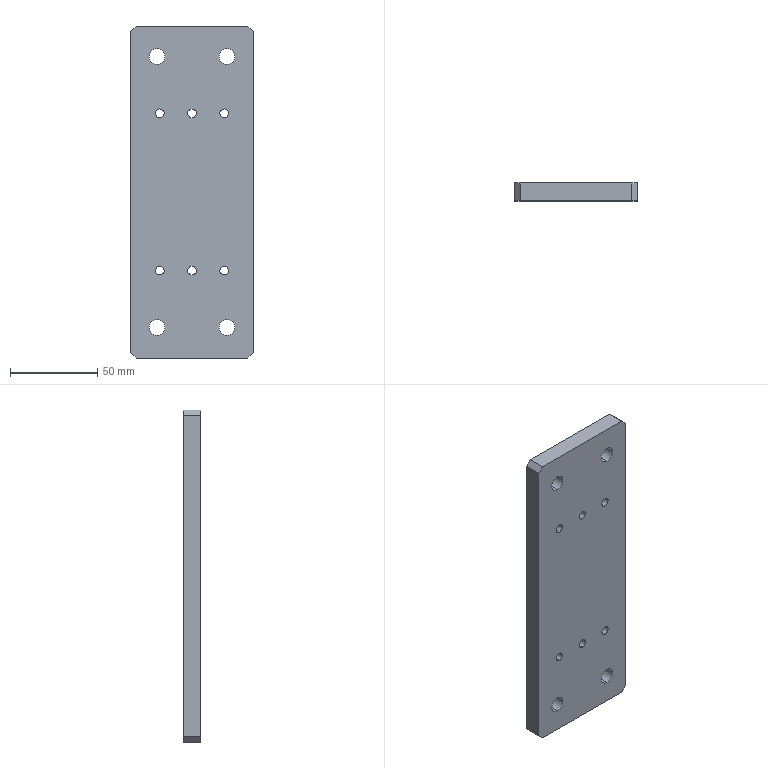Part | SolidWorks | features HoleWzd 2, Chamfer 1, Extrusion 1 | 1 solid | 30 faces | box 70 x 10 x 190 mm | volume 129097 mm3 | cylinder 20 | plane 10 | commonest cylinder face diameters 5 x12 9 x8
STEP:
#1=CARTESIAN_POINT('',(-20.,0.,-82.));
#2=VERTEX_POINT('',#1);
#3=CARTESIAN_POINT('',(-20.,0.,-73.));
#4=VERTEX_POINT('',#3);
#5=CARTESIAN_POINT('',(-20.,0.,-77.5));
#6=DIRECTION('',(0.,1.,0.));
#7=DIRECTION('',(0.,0.,1.));
#8=AXIS2_PLACEMENT_3D('',#5,#6,#7);
#9=CIRCLE('',#8,4.5);
#10=EDGE_CURVE('',#2,#4,#9,.T.);
#11=ORIENTED_EDGE('',*,*,#10,.F.);
#12=CARTESIAN_POINT('',(-20.,10.,-82.));
#13=VERTEX_POINT('',#12);
#14=CARTESIAN_POINT('',(-20.,10.,-82.));
#15=DIRECTION('',(0.,1.,0.));
#16=VECTOR('',#15,1000.);
#17=LINE('',#14,#16);
#18=EDGE_CURVE('',#2,#13,#17,.T.);
#19=ORIENTED_EDGE('',*,*,#18,.T.);
#20=CARTESIAN_POINT('',(-20.,10.,-73.));
#21=VERTEX_POINT('',#20);
#22=CARTESIAN_POINT('',(-20.,10.,-77.5));
#23=DIRECTION('',(0.,1.,0.));
#24=DIRECTION('',(0.,0.,1.));
#25=AXIS2_PLACEMENT_3D('',#22,#23,#24);
#26=CIRCLE('',#25,4.5);
#27=EDGE_CURVE('',#13,#21,#26,.T.);
#28=ORIENTED_EDGE('',*,*,#27,.T.);
#29=CARTESIAN_POINT('',(-20.,10.,-73.));
#30=DIRECTION('',(0.,1.,0.));
#31=VECTOR('',#30,1000.);
#32=LINE('',#29,#31);
#33=EDGE_CURVE('',#4,#21,#32,.T.);
#34=ORIENTED_EDGE('',*,*,#33,.F.);
#35=EDGE_LOOP('',(#11,#19,#28,#34));
#36=FACE_OUTER_BOUND('',#35,.T.);
#37=CARTESIAN_POINT('',(-20.,10.,-77.5));
#38=DIRECTION('',(0.,1.,0.));
#39=DIRECTION('',(0.,0.,1.));
#40=AXIS2_PLACEMENT_3D('',#37,#38,#39);
#41=CYLINDRICAL_SURFACE('',#40,4.5);
#42=ADVANCED_FACE('',(#36),#41,.F.);
#43=CARTESIAN_POINT('',(20.,0.,-82.));
#44=VERTEX_POINT('',#43);
#45=CARTESIAN_POINT('',(20.,0.,-73.));
#46=VERTEX_POINT('',#45);
#47=CARTESIAN_POINT('',(20.,0.,-77.5));
#48=DIRECTION('',(0.,1.,0.));
#49=DIRECTION('',(0.,0.,1.));
#50=AXIS2_PLACEMENT_3D('',#47,#48,#49);
#51=CIRCLE('',#50,4.5);
#52=EDGE_CURVE('',#44,#46,#51,.T.);
#53=ORIENTED_EDGE('',*,*,#52,.F.);
#54=CARTESIAN_POINT('',(20.,10.,-82.));
#55=VERTEX_POINT('',#54);
#56=CARTESIAN_POINT('',(20.,10.,-82.));
#57=DIRECTION('',(0.,1.,0.));
#58=VECTOR('',#57,1000.);
#59=LINE('',#56,#58);
#60=EDGE_CURVE('',#44,#55,#59,.T.);
#61=ORIENTED_EDGE('',*,*,#60,.T.);
#62=CARTESIAN_POINT('',(20.,10.,-73.));
#63=VERTEX_POINT('',#62);
#64=CARTESIAN_POINT('',(20.,10.,-77.5));
#65=DIRECTION('',(0.,1.,0.));
#66=DIRECTION('',(0.,0.,1.));
#67=AXIS2_PLACEMENT_3D('',#64,#65,#66);
#68=CIRCLE('',#67,4.5);
#69=EDGE_CURVE('',#55,#63,#68,.T.);
#70=ORIENTED_EDGE('',*,*,#69,.T.);
#71=CARTESIAN_POINT('',(20.,10.,-73.));
#72=DIRECTION('',(0.,1.,0.));
#73=VECTOR('',#72,1000.);
#74=LINE('',#71,#73);
#75=EDGE_CURVE('',#46,#63,#74,.T.);
#76=ORIENTED_EDGE('',*,*,#75,.F.);
#77=EDGE_LOOP('',(#53,#61,#70,#76));
#78=FACE_OUTER_BOUND('',#77,.T.);
#79=CARTESIAN_POINT('',(20.,10.,-77.5));
#80=DIRECTION('',(0.,1.,0.));
#81=DIRECTION('',(0.,0.,1.));
#82=AXIS2_PLACEMENT_3D('',#79,#80,#81);
#83=CYLINDRICAL_SURFACE('',#82,4.5);
#84=ADVANCED_FACE('',(#78),#83,.F.);
#85=CARTESIAN_POINT('',(20.,0.,73.));
#86=VERTEX_POINT('',#85);
#87=CARTESIAN_POINT('',(20.,0.,82.));
#88=VERTEX_POINT('',#87);
#89=CARTESIAN_POINT('',(20.,0.,77.5));
#90=DIRECTION('',(0.,1.,0.));
#91=DIRECTION('',(0.,0.,1.));
#92=AXIS2_PLACEMENT_3D('',#89,#90,#91);
#93=CIRCLE('',#92,4.5);
#94=EDGE_CURVE('',#86,#88,#93,.T.);
#95=ORIENTED_EDGE('',*,*,#94,.F.);
#96=CARTESIAN_POINT('',(20.,10.,73.));
#97=VERTEX_POINT('',#96);
#98=CARTESIAN_POINT('',(20.,10.,73.));
#99=DIRECTION('',(0.,1.,0.));
#100=VECTOR('',#99,1000.);
#101=LINE('',#98,#100);
#102=EDGE_CURVE('',#86,#97,#101,.T.);
#103=ORIENTED_EDGE('',*,*,#102,.T.);
#104=CARTESIAN_POINT('',(20.,10.,82.));
#105=VERTEX_POINT('',#104);
#106=CARTESIAN_POINT('',(20.,10.,77.5));
#107=DIRECTION('',(0.,1.,0.));
#108=DIRECTION('',(0.,0.,1.));
#109=AXIS2_PLACEMENT_3D('',#106,#107,#108);
#110=CIRCLE('',#109,4.5);
#111=EDGE_CURVE('',#97,#105,#110,.T.);
#112=ORIENTED_EDGE('',*,*,#111,.T.);
#113=CARTESIAN_POINT('',(20.,10.,82.));
#114=DIRECTION('',(0.,1.,0.));
#115=VECTOR('',#114,1000.);
#116=LINE('',#113,#115);
#117=EDGE_CURVE('',#88,#105,#116,.T.);
#118=ORIENTED_EDGE('',*,*,#117,.F.);
#119=EDGE_LOOP('',(#95,#103,#112,#118));
#120=FACE_OUTER_BOUND('',#119,.T.);
#121=CARTESIAN_POINT('',(20.,10.,77.5));
#122=DIRECTION('',(0.,1.,0.));
#123=DIRECTION('',(0.,0.,1.));
#124=AXIS2_PLACEMENT_3D('',#121,#122,#123);
#125=CYLINDRICAL_SURFACE('',#124,4.5);
#126=ADVANCED_FACE('',(#120),#125,.F.);
#127=CARTESIAN_POINT('',(-20.,0.,73.));
#128=VERTEX_POINT('',#127);
#129=CARTESIAN_POINT('',(-20.,0.,82.));
#130=VERTEX_POINT('',#129);
#131=CARTESIAN_POINT('',(-20.,0.,77.5));
#132=DIRECTION('',(0.,1.,0.));
#133=DIRECTION('',(0.,0.,1.));
#134=AXIS2_PLACEMENT_3D('',#131,#132,#133);
#135=CIRCLE('',#134,4.5);
#136=EDGE_CURVE('',#128,#130,#135,.T.);
#137=ORIENTED_EDGE('',*,*,#136,.F.);
#138=CARTESIAN_POINT('',(-20.,10.,73.));
#139=VERTEX_POINT('',#138);
#140=CARTESIAN_POINT('',(-20.,10.,73.));
#141=DIRECTION('',(0.,1.,0.));
#142=VECTOR('',#141,1000.);
#143=LINE('',#140,#142);
#144=EDGE_CURVE('',#128,#139,#143,.T.);
#145=ORIENTED_EDGE('',*,*,#144,.T.);
#146=CARTESIAN_POINT('',(-20.,10.,82.));
#147=VERTEX_POINT('',#146);
#148=CARTESIAN_POINT('',(-20.,10.,77.5));
#149=DIRECTION('',(0.,1.,0.));
#150=DIRECTION('',(0.,0.,1.));
#151=AXIS2_PLACEMENT_3D('',#148,#149,#150);
#152=CIRCLE('',#151,4.5);
#153=EDGE_CURVE('',#139,#147,#152,.T.);
#154=ORIENTED_EDGE('',*,*,#153,.T.);
#155=CARTESIAN_POINT('',(-20.,10.,82.));
#156=DIRECTION('',(0.,1.,0.));
#157=VECTOR('',#156,1000.);
#158=LINE('',#155,#157);
#159=EDGE_CURVE('',#130,#147,#158,.T.);
#160=ORIENTED_EDGE('',*,*,#159,.F.);
#161=EDGE_LOOP('',(#137,#145,#154,#160));
#162=FACE_OUTER_BOUND('',#161,.T.);
#163=CARTESIAN_POINT('',(-20.,10.,77.5));
#164=DIRECTION('',(0.,1.,0.));
#165=DIRECTION('',(0.,0.,1.));
#166=AXIS2_PLACEMENT_3D('',#163,#164,#165);
#167=CYLINDRICAL_SURFACE('',#166,4.5);
#168=ADVANCED_FACE('',(#162),#167,.F.);
#169=CARTESIAN_POINT('',(18.5,0.,-47.5));
#170=VERTEX_POINT('',#169);
#171=CARTESIAN_POINT('',(18.5,0.,-42.5));
#172=VERTEX_POINT('',#171);
#173=CARTESIAN_POINT('',(18.5,0.,-45.));
#174=DIRECTION('',(0.,1.,0.));
#175=DIRECTION('',(0.,0.,1.));
#176=AXIS2_PLACEMENT_3D('',#173,#174,#175);
#177=CIRCLE('',#176,2.5);
#178=EDGE_CURVE('',#170,#172,#177,.T.);
#179=ORIENTED_EDGE('',*,*,#178,.F.);
#180=CARTESIAN_POINT('',(18.5,10.,-47.5));
#181=VERTEX_POINT('',#180);
#182=CARTESIAN_POINT('',(18.5,10.,-47.5));
#183=DIRECTION('',(0.,1.,0.));
#184=VECTOR('',#183,1000.);
#185=LINE('',#182,#184);
#186=EDGE_CURVE('',#170,#181,#185,.T.);
#187=ORIENTED_EDGE('',*,*,#186,.T.);
#188=CARTESIAN_POINT('',(18.5,10.,-42.5));
#189=VERTEX_POINT('',#188);
#190=CARTESIAN_POINT('',(18.5,10.,-45.));
#191=DIRECTION('',(0.,1.,0.));
#192=DIRECTION('',(0.,0.,1.));
#193=AXIS2_PLACEMENT_3D('',#190,#191,#192);
#194=CIRCLE('',#193,2.5);
#195=EDGE_CURVE('',#181,#189,#194,.T.);
#196=ORIENTED_EDGE('',*,*,#195,.T.);
#197=CARTESIAN_POINT('',(18.5,10.,-42.5));
#198=DIRECTION('',(0.,1.,0.));
#199=VECTOR('',#198,1000.);
#200=LINE('',#197,#199);
#201=EDGE_CURVE('',#172,#189,#200,.T.);
#202=ORIENTED_EDGE('',*,*,#201,.F.);
#203=EDGE_LOOP('',(#179,#187,#196,#202));
#204=FACE_OUTER_BOUND('',#203,.T.);
#205=CARTESIAN_POINT('',(18.5,10.,-45.));
#206=DIRECTION('',(0.,1.,0.));
#207=DIRECTION('',(0.,0.,1.));
#208=AXIS2_PLACEMENT_3D('',#205,#206,#207);
#209=CYLINDRICAL_SURFACE('',#208,2.5);
#210=ADVANCED_FACE('',(#204),#209,.F.);
#211=CARTESIAN_POINT('',(-18.5,0.,-47.5));
#212=VERTEX_POINT('',#211);
#213=CARTESIAN_POINT('',(-18.5,0.,-42.5));
#214=VERTEX_POINT('',#213);
#215=CARTESIAN_POINT('',(-18.5,0.,-45.));
#216=DIRECTION('',(0.,1.,0.));
#217=DIRECTION('',(0.,0.,1.));
#218=AXIS2_PLACEMENT_3D('',#215,#216,#217);
#219=CIRCLE('',#218,2.5);
#220=EDGE_CURVE('',#212,#214,#219,.T.);
#221=ORIENTED_EDGE('',*,*,#220,.F.);
#222=CARTESIAN_POINT('',(-18.5,10.,-47.5));
#223=VERTEX_POINT('',#222);
#224=CARTESIAN_POINT('',(-18.5,10.,-47.5));
#225=DIRECTION('',(0.,1.,0.));
#226=VECTOR('',#225,1000.);
#227=LINE('',#224,#226);
#228=EDGE_CURVE('',#212,#223,#227,.T.);
#229=ORIENTED_EDGE('',*,*,#228,.T.);
#230=CARTESIAN_POINT('',(-18.5,10.,-42.5));
#231=VERTEX_POINT('',#230);
#232=CARTESIAN_POINT('',(-18.5,10.,-45.));
#233=DIRECTION('',(0.,1.,0.));
#234=DIRECTION('',(0.,0.,1.));
#235=AXIS2_PLACEMENT_3D('',#232,#233,#234);
#236=CIRCLE('',#235,2.5);
#237=EDGE_CURVE('',#223,#231,#236,.T.);
#238=ORIENTED_EDGE('',*,*,#237,.T.);
#239=CARTESIAN_POINT('',(-18.5,10.,-42.5));
#240=DIRECTION('',(0.,1.,0.));
#241=VECTOR('',#240,1000.);
#242=LINE('',#239,#241);
#243=EDGE_CURVE('',#214,#231,#242,.T.);
#244=ORIENTED_EDGE('',*,*,#243,.F.);
#245=EDGE_LOOP('',(#221,#229,#238,#244));
#246=FACE_OUTER_BOUND('',#245,.T.);
#247=CARTESIAN_POINT('',(-18.5,10.,-45.));
#248=DIRECTION('',(0.,1.,0.));
#249=DIRECTION('',(0.,0.,1.));
#250=AXIS2_PLACEMENT_3D('',#247,#248,#249);
#251=CYLINDRICAL_SURFACE('',#250,2.5);
#252=ADVANCED_FACE('',(#246),#251,.F.);
#253=CARTESIAN_POINT('',(0.,0.,-47.5));
#254=VERTEX_POINT('',#253);
#255=CARTESIAN_POINT('',(0.,0.,-42.5));
#256=VERTEX_POINT('',#255);
#257=CARTESIAN_POINT('',(0.,0.,-45.));
#258=DIRECTION('',(0.,1.,0.));
#259=DIRECTION('',(0.,0.,1.));
#260=AXIS2_PLACEMENT_3D('',#257,#258,#259);
#261=CIRCLE('',#260,2.5);
#262=EDGE_CURVE('',#254,#256,#261,.T.);
#263=ORIENTED_EDGE('',*,*,#262,.F.);
#264=CARTESIAN_POINT('',(0.,10.,-47.5));
#265=VERTEX_POINT('',#264);
#266=CARTESIAN_POINT('',(0.,10.,-47.5));
#267=DIRECTION('',(0.,1.,0.));
#268=VECTOR('',#267,1000.);
#269=LINE('',#266,#268);
#270=EDGE_CURVE('',#254,#265,#269,.T.);
#271=ORIENTED_EDGE('',*,*,#270,.T.);
#272=CARTESIAN_POINT('',(0.,10.,-42.5));
#273=VERTEX_POINT('',#272);
#274=CARTESIAN_POINT('',(0.,10.,-45.));
#275=DIRECTION('',(0.,1.,0.));
#276=DIRECTION('',(0.,0.,1.));
#277=AXIS2_PLACEMENT_3D('',#274,#275,#276);
#278=CIRCLE('',#277,2.5);
#279=EDGE_CURVE('',#265,#273,#278,.T.);
#280=ORIENTED_EDGE('',*,*,#279,.T.);
#281=CARTESIAN_POINT('',(0.,10.,-42.5));
#282=DIRECTION('',(0.,1.,0.));
#283=VECTOR('',#282,1000.);
#284=LINE('',#281,#283);
#285=EDGE_CURVE('',#256,#273,#284,.T.);
#286=ORIENTED_EDGE('',*,*,#285,.F.);
#287=EDGE_LOOP('',(#263,#271,#280,#286));
#288=FACE_OUTER_BOUND('',#287,.T.);
#289=CARTESIAN_POINT('',(0.,10.,-45.));
#290=DIRECTION('',(0.,1.,0.));
#291=DIRECTION('',(0.,0.,1.));
#292=AXIS2_PLACEMENT_3D('',#289,#290,#291);
#293=CYLINDRICAL_SURFACE('',#292,2.5);
#294=ADVANCED_FACE('',(#288),#293,.F.);
#295=CARTESIAN_POINT('',(0.,0.,42.5));
#296=VERTEX_POINT('',#295);
#297=CARTESIAN_POINT('',(0.,0.,47.5));
#298=VERTEX_POINT('',#297);
#299=CARTESIAN_POINT('',(0.,0.,45.));
#300=DIRECTION('',(0.,1.,0.));
#301=DIRECTION('',(0.,0.,1.));
#302=AXIS2_PLACEMENT_3D('',#299,#300,#301);
#303=CIRCLE('',#302,2.5);
#304=EDGE_CURVE('',#296,#298,#303,.T.);
#305=ORIENTED_EDGE('',*,*,#304,.F.);
#306=CARTESIAN_POINT('',(0.,10.,42.5));
#307=VERTEX_POINT('',#306);
#308=CARTESIAN_POINT('',(0.,10.,42.5));
#309=DIRECTION('',(0.,1.,0.));
#310=VECTOR('',#309,1000.);
#311=LINE('',#308,#310);
#312=EDGE_CURVE('',#296,#307,#311,.T.);
#313=ORIENTED_EDGE('',*,*,#312,.T.);
#314=CARTESIAN_POINT('',(0.,10.,47.5));
#315=VERTEX_POINT('',#314);
#316=CARTESIAN_POINT('',(0.,10.,45.));
#317=DIRECTION('',(0.,1.,0.));
#318=DIRECTION('',(0.,0.,1.));
#319=AXIS2_PLACEMENT_3D('',#316,#317,#318);
#320=CIRCLE('',#319,2.5);
#321=EDGE_CURVE('',#307,#315,#320,.T.);
#322=ORIENTED_EDGE('',*,*,#321,.T.);
#323=CARTESIAN_POINT('',(0.,10.,47.5));
#324=DIRECTION('',(0.,1.,0.));
#325=VECTOR('',#324,1000.);
#326=LINE('',#323,#325);
#327=EDGE_CURVE('',#298,#315,#326,.T.);
#328=ORIENTED_EDGE('',*,*,#327,.F.);
#329=EDGE_LOOP('',(#305,#313,#322,#328));
#330=FACE_OUTER_BOUND('',#329,.T.);
#331=CARTESIAN_POINT('',(0.,10.,45.));
#332=DIRECTION('',(0.,1.,0.));
#333=DIRECTION('',(0.,0.,1.));
#334=AXIS2_PLACEMENT_3D('',#331,#332,#333);
#335=CYLINDRICAL_SURFACE('',#334,2.5);
#336=ADVANCED_FACE('',(#330),#335,.F.);
#337=CARTESIAN_POINT('',(-18.5,0.,42.5));
#338=VERTEX_POINT('',#337);
#339=CARTESIAN_POINT('',(-18.5,0.,47.5));
#340=VERTEX_POINT('',#339);
#341=CARTESIAN_POINT('',(-18.5,0.,45.));
#342=DIRECTION('',(0.,1.,0.));
#343=DIRECTION('',(0.,0.,1.));
#344=AXIS2_PLACEMENT_3D('',#341,#342,#343);
#345=CIRCLE('',#344,2.5);
#346=EDGE_CURVE('',#338,#340,#345,.T.);
#347=ORIENTED_EDGE('',*,*,#346,.F.);
#348=CARTESIAN_POINT('',(-18.5,10.,42.5));
#349=VERTEX_POINT('',#348);
#350=CARTESIAN_POINT('',(-18.5,10.,42.5));
#351=DIRECTION('',(0.,1.,0.));
#352=VECTOR('',#351,1000.);
#353=LINE('',#350,#352);
#354=EDGE_CURVE('',#338,#349,#353,.T.);
#355=ORIENTED_EDGE('',*,*,#354,.T.);
#356=CARTESIAN_POINT('',(-18.5,10.,47.5));
#357=VERTEX_POINT('',#356);
#358=CARTESIAN_POINT('',(-18.5,10.,45.));
#359=DIRECTION('',(0.,1.,0.));
#360=DIRECTION('',(0.,0.,1.));
#361=AXIS2_PLACEMENT_3D('',#358,#359,#360);
#362=CIRCLE('',#361,2.5);
#363=EDGE_CURVE('',#349,#357,#362,.T.);
#364=ORIENTED_EDGE('',*,*,#363,.T.);
#365=CARTESIAN_POINT('',(-18.5,10.,47.5));
#366=DIRECTION('',(0.,1.,0.));
#367=VECTOR('',#366,1000.);
#368=LINE('',#365,#367);
#369=EDGE_CURVE('',#340,#357,#368,.T.);
#370=ORIENTED_EDGE('',*,*,#369,.F.);
#371=EDGE_LOOP('',(#347,#355,#364,#370));
#372=FACE_OUTER_BOUND('',#371,.T.);
#373=CARTESIAN_POINT('',(-18.5,10.,45.));
#374=DIRECTION('',(0.,1.,0.));
#375=DIRECTION('',(0.,0.,1.));
#376=AXIS2_PLACEMENT_3D('',#373,#374,#375);
#377=CYLINDRICAL_SURFACE('',#376,2.5);
#378=ADVANCED_FACE('',(#372),#377,.F.);
#379=CARTESIAN_POINT('',(18.5,0.,42.5));
#380=VERTEX_POINT('',#379);
#381=CARTESIAN_POINT('',(18.5,0.,47.5));
#382=VERTEX_POINT('',#381);
#383=CARTESIAN_POINT('',(18.5,0.,45.));
#384=DIRECTION('',(0.,1.,0.));
#385=DIRECTION('',(0.,0.,1.));
#386=AXIS2_PLACEMENT_3D('',#383,#384,#385);
#387=CIRCLE('',#386,2.5);
#388=EDGE_CURVE('',#380,#382,#387,.T.);
#389=ORIENTED_EDGE('',*,*,#388,.F.);
#390=CARTESIAN_POINT('',(18.5,10.,42.5));
#391=VERTEX_POINT('',#390);
#392=CARTESIAN_POINT('',(18.5,10.,42.5));
#393=DIRECTION('',(0.,1.,0.));
#394=VECTOR('',#393,1000.);
#395=LINE('',#392,#394);
#396=EDGE_CURVE('',#380,#391,#395,.T.);
#397=ORIENTED_EDGE('',*,*,#396,.T.);
#398=CARTESIAN_POINT('',(18.5,10.,47.5));
#399=VERTEX_POINT('',#398);
#400=CARTESIAN_POINT('',(18.5,10.,45.));
#401=DIRECTION('',(0.,1.,0.));
#402=DIRECTION('',(0.,0.,1.));
#403=AXIS2_PLACEMENT_3D('',#400,#401,#402);
#404=CIRCLE('',#403,2.5);
#405=EDGE_CURVE('',#391,#399,#404,.T.);
#406=ORIENTED_EDGE('',*,*,#405,.T.);
#407=CARTESIAN_POINT('',(18.5,10.,47.5));
#408=DIRECTION('',(0.,1.,0.));
#409=VECTOR('',#408,1000.);
#410=LINE('',#407,#409);
#411=EDGE_CURVE('',#382,#399,#410,.T.);
#412=ORIENTED_EDGE('',*,*,#411,.F.);
#413=EDGE_LOOP('',(#389,#397,#406,#412));
#414=FACE_OUTER_BOUND('',#413,.T.);
#415=CARTESIAN_POINT('',(18.5,10.,45.));
#416=DIRECTION('',(0.,1.,0.));
#417=DIRECTION('',(0.,0.,1.));
#418=AXIS2_PLACEMENT_3D('',#415,#416,#417);
#419=CYLINDRICAL_SURFACE('',#418,2.5);
#420=ADVANCED_FACE('',(#414),#419,.F.);
#421=CARTESIAN_POINT('',(35.,0.,92.));
#422=VERTEX_POINT('',#421);
#423=CARTESIAN_POINT('',(35.,0.,-92.));
#424=VERTEX_POINT('',#423);
#425=CARTESIAN_POINT('',(35.,0.,-95.));
#426=DIRECTION('',(0.,0.,-1.));
#427=VECTOR('',#426,1000.);
#428=LINE('',#425,#427);
#429=EDGE_CURVE('',#422,#424,#428,.T.);
#430=ORIENTED_EDGE('',*,*,#429,.T.);
#431=CARTESIAN_POINT('',(35.,10.,-92.));
#432=VERTEX_POINT('',#431);
#433=CARTESIAN_POINT('',(35.,10.,-92.));
#434=DIRECTION('',(0.,1.,0.));
#435=VECTOR('',#434,1000.);
#436=LINE('',#433,#435);
#437=EDGE_CURVE('',#424,#432,#436,.T.);
#438=ORIENTED_EDGE('',*,*,#437,.T.);
#439=CARTESIAN_POINT('',(35.,10.,92.));
#440=VERTEX_POINT('',#439);
#441=CARTESIAN_POINT('',(35.,10.,-95.));
#442=DIRECTION('',(0.,0.,-1.));
#443=VECTOR('',#442,1000.);
#444=LINE('',#441,#443);
#445=EDGE_CURVE('',#440,#432,#444,.T.);
#446=ORIENTED_EDGE('',*,*,#445,.F.);
#447=CARTESIAN_POINT('',(35.,10.,92.));
#448=DIRECTION('',(0.,-1.,0.));
#449=VECTOR('',#448,1000.);
#450=LINE('',#447,#449);
#451=EDGE_CURVE('',#440,#422,#450,.T.);
#452=ORIENTED_EDGE('',*,*,#451,.T.);
#453=EDGE_LOOP('',(#430,#438,#446,#452));
#454=FACE_OUTER_BOUND('',#453,.T.);
#455=CARTESIAN_POINT('',(35.,10.,-95.));
#456=DIRECTION('',(-1.,0.,0.));
#457=DIRECTION('',(0.,0.,1.));
#458=AXIS2_PLACEMENT_3D('',#455,#456,#457);
#459=PLANE('',#458);
#460=ADVANCED_FACE('',(#454),#459,.F.);
#461=CARTESIAN_POINT('',(32.,0.,-95.));
#462=VERTEX_POINT('',#461);
#463=CARTESIAN_POINT('',(-32.,0.,-95.));
#464=VERTEX_POINT('',#463);
#465=CARTESIAN_POINT('',(-35.,0.,-95.));
#466=DIRECTION('',(-1.,0.,0.));
#467=VECTOR('',#466,1000.);
#468=LINE('',#465,#467);
#469=EDGE_CURVE('',#462,#464,#468,.T.);
#470=ORIENTED_EDGE('',*,*,#469,.T.);
#471=CARTESIAN_POINT('',(-32.,10.,-95.));
#472=VERTEX_POINT('',#471);
#473=CARTESIAN_POINT('',(-32.,10.,-95.));
#474=DIRECTION('',(0.,1.,0.));
#475=VECTOR('',#474,1000.);
#476=LINE('',#473,#475);
#477=EDGE_CURVE('',#464,#472,#476,.T.);
#478=ORIENTED_EDGE('',*,*,#477,.T.);
#479=CARTESIAN_POINT('',(32.,10.,-95.));
#480=VERTEX_POINT('',#479);
#481=CARTESIAN_POINT('',(-35.,10.,-95.));
#482=DIRECTION('',(-1.,0.,0.));
#483=VECTOR('',#482,1000.);
#484=LINE('',#481,#483);
#485=EDGE_CURVE('',#480,#472,#484,.T.);
#486=ORIENTED_EDGE('',*,*,#485,.F.);
#487=CARTESIAN_POINT('',(32.,10.,-95.));
#488=DIRECTION('',(0.,-1.,0.));
#489=VECTOR('',#488,1000.);
#490=LINE('',#487,#489);
#491=EDGE_CURVE('',#480,#462,#490,.T.);
#492=ORIENTED_EDGE('',*,*,#491,.T.);
#493=EDGE_LOOP('',(#470,#478,#486,#492));
#494=FACE_OUTER_BOUND('',#493,.T.);
#495=CARTESIAN_POINT('',(-35.,10.,-95.));
#496=DIRECTION('',(0.,0.,1.));
#497=DIRECTION('',(1.,0.,0.));
#498=AXIS2_PLACEMENT_3D('',#495,#496,#497);
#499=PLANE('',#498);
#500=ADVANCED_FACE('',(#494),#499,.F.);
#501=CARTESIAN_POINT('',(-35.,10.,-92.));
#502=VERTEX_POINT('',#501);
#503=CARTESIAN_POINT('',(-35.,10.,92.));
#504=VERTEX_POINT('',#503);
#505=CARTESIAN_POINT('',(-35.,10.,-95.));
#506=DIRECTION('',(0.,0.,1.));
#507=VECTOR('',#506,1000.);
#508=LINE('',#505,#507);
#509=EDGE_CURVE('',#502,#504,#508,.T.);
#510=ORIENTED_EDGE('',*,*,#509,.F.);
#511=CARTESIAN_POINT('',(-35.,0.,-92.));
#512=VERTEX_POINT('',#511);
#513=CARTESIAN_POINT('',(-35.,10.,-92.));
#514=DIRECTION('',(0.,-1.,0.));
#515=VECTOR('',#514,1000.);
#516=LINE('',#513,#515);
#517=EDGE_CURVE('',#502,#512,#516,.T.);
#518=ORIENTED_EDGE('',*,*,#517,.T.);
#519=CARTESIAN_POINT('',(-35.,0.,92.));
#520=VERTEX_POINT('',#519);
#521=CARTESIAN_POINT('',(-35.,0.,-95.));
#522=DIRECTION('',(0.,0.,1.));
#523=VECTOR('',#522,1000.);
#524=LINE('',#521,#523);
#525=EDGE_CURVE('',#512,#520,#524,.T.);
#526=ORIENTED_EDGE('',*,*,#525,.T.);
#527=CARTESIAN_POINT('',(-35.,10.,92.));
#528=DIRECTION('',(0.,1.,0.));
#529=VECTOR('',#528,1000.);
#530=LINE('',#527,#529);
#531=EDGE_CURVE('',#520,#504,#530,.T.);
#532=ORIENTED_EDGE('',*,*,#531,.T.);
#533=EDGE_LOOP('',(#510,#518,#526,#532));
#534=FACE_OUTER_BOUND('',#533,.T.);
#535=CARTESIAN_POINT('',(-35.,10.,-95.));
#536=DIRECTION('',(1.,0.,0.));
#537=DIRECTION('',(0.,0.,-1.));
#538=AXIS2_PLACEMENT_3D('',#535,#536,#537);
#539=PLANE('',#538);
#540=ADVANCED_FACE('',(#534),#539,.F.);
#541=CARTESIAN_POINT('',(-32.,10.,95.));
#542=VERTEX_POINT('',#541);
#543=CARTESIAN_POINT('',(32.,10.,95.));
#544=VERTEX_POINT('',#543);
#545=CARTESIAN_POINT('',(-35.,10.,95.));
#546=DIRECTION('',(1.,0.,0.));
#547=VECTOR('',#546,1000.);
#548=LINE('',#545,#547);
#549=EDGE_CURVE('',#542,#544,#548,.T.);
#550=ORIENTED_EDGE('',*,*,#549,.F.);
#551=CARTESIAN_POINT('',(-32.,0.,95.));
#552=VERTEX_POINT('',#551);
#553=CARTESIAN_POINT('',(-32.,10.,95.));
#554=DIRECTION('',(0.,-1.,0.));
#555=VECTOR('',#554,1000.);
#556=LINE('',#553,#555);
#557=EDGE_CURVE('',#542,#552,#556,.T.);
#558=ORIENTED_EDGE('',*,*,#557,.T.);
#559=CARTESIAN_POINT('',(32.,0.,95.));
#560=VERTEX_POINT('',#559);
#561=CARTESIAN_POINT('',(-35.,0.,95.));
#562=DIRECTION('',(1.,0.,0.));
#563=VECTOR('',#562,1000.);
#564=LINE('',#561,#563);
#565=EDGE_CURVE('',#552,#560,#564,.T.);
#566=ORIENTED_EDGE('',*,*,#565,.T.);
#567=CARTESIAN_POINT('',(32.,10.,95.));
#568=DIRECTION('',(0.,1.,0.));
#569=VECTOR('',#568,1000.);
#570=LINE('',#567,#569);
#571=EDGE_CURVE('',#560,#544,#570,.T.);
#572=ORIENTED_EDGE('',*,*,#571,.T.);
#573=EDGE_LOOP('',(#550,#558,#566,#572));
#574=FACE_OUTER_BOUND('',#573,.T.);
#575=CARTESIAN_POINT('',(-35.,10.,95.));
#576=DIRECTION('',(0.,0.,-1.));
#577=DIRECTION('',(-1.,0.,0.));
#578=AXIS2_PLACEMENT_3D('',#575,#576,#577);
#579=PLANE('',#578);
#580=ADVANCED_FACE('',(#574),#579,.F.);
#581=CARTESIAN_POINT('',(-20.,10.,-77.5));
#582=DIRECTION('',(0.,1.,0.));
#583=DIRECTION('',(0.,0.,1.));
#584=AXIS2_PLACEMENT_3D('',#581,#582,#583);
#585=CIRCLE('',#584,4.5);
#586=EDGE_CURVE('',#21,#13,#585,.T.);
#587=ORIENTED_EDGE('',*,*,#586,.F.);
#588=ORIENTED_EDGE('',*,*,#27,.F.);
#589=EDGE_LOOP('',(#587,#588));
#590=FACE_BOUND('',#589,.T.);
#591=CARTESIAN_POINT('',(20.,10.,-77.5));
#592=DIRECTION('',(0.,1.,0.));
#593=DIRECTION('',(0.,0.,1.));
#594=AXIS2_PLACEMENT_3D('',#591,#592,#593);
#595=CIRCLE('',#594,4.5);
#596=EDGE_CURVE('',#63,#55,#595,.T.);
#597=ORIENTED_EDGE('',*,*,#596,.F.);
#598=ORIENTED_EDGE('',*,*,#69,.F.);
#599=EDGE_LOOP('',(#597,#598));
#600=FACE_BOUND('',#599,.T.);
#601=CARTESIAN_POINT('',(20.,10.,77.5));
#602=DIRECTION('',(0.,1.,0.));
#603=DIRECTION('',(0.,0.,1.));
#604=AXIS2_PLACEMENT_3D('',#601,#602,#603);
#605=CIRCLE('',#604,4.5);
#606=EDGE_CURVE('',#105,#97,#605,.T.);
#607=ORIENTED_EDGE('',*,*,#606,.F.);
#608=ORIENTED_EDGE('',*,*,#111,.F.);
#609=EDGE_LOOP('',(#607,#608));
#610=FACE_BOUND('',#609,.T.);
#611=CARTESIAN_POINT('',(-20.,10.,77.5));
#612=DIRECTION('',(0.,1.,0.));
#613=DIRECTION('',(0.,0.,1.));
#614=AXIS2_PLACEMENT_3D('',#611,#612,#613);
#615=CIRCLE('',#614,4.5);
#616=EDGE_CURVE('',#147,#139,#615,.T.);
#617=ORIENTED_EDGE('',*,*,#616,.F.);
#618=ORIENTED_EDGE('',*,*,#153,.F.);
#619=EDGE_LOOP('',(#617,#618));
#620=FACE_BOUND('',#619,.T.);
#621=CARTESIAN_POINT('',(18.5,10.,-45.));
#622=DIRECTION('',(0.,1.,0.));
#623=DIRECTION('',(0.,0.,1.));
#624=AXIS2_PLACEMENT_3D('',#621,#622,#623);
#625=CIRCLE('',#624,2.5);
#626=EDGE_CURVE('',#189,#181,#625,.T.);
#627=ORIENTED_EDGE('',*,*,#626,.F.);
#628=ORIENTED_EDGE('',*,*,#195,.F.);
#629=EDGE_LOOP('',(#627,#628));
#630=FACE_BOUND('',#629,.T.);
#631=CARTESIAN_POINT('',(-18.5,10.,-45.));
#632=DIRECTION('',(0.,1.,0.));
#633=DIRECTION('',(0.,0.,1.));
#634=AXIS2_PLACEMENT_3D('',#631,#632,#633);
#635=CIRCLE('',#634,2.5);
#636=EDGE_CURVE('',#231,#223,#635,.T.);
#637=ORIENTED_EDGE('',*,*,#636,.F.);
#638=ORIENTED_EDGE('',*,*,#237,.F.);
#639=EDGE_LOOP('',(#637,#638));
#640=FACE_BOUND('',#639,.T.);
#641=CARTESIAN_POINT('',(0.,10.,-45.));
#642=DIRECTION('',(0.,1.,0.));
#643=DIRECTION('',(0.,0.,1.));
#644=AXIS2_PLACEMENT_3D('',#641,#642,#643);
#645=CIRCLE('',#644,2.5);
#646=EDGE_CURVE('',#273,#265,#645,.T.);
#647=ORIENTED_EDGE('',*,*,#646,.F.);
#648=ORIENTED_EDGE('',*,*,#279,.F.);
#649=EDGE_LOOP('',(#647,#648));
#650=FACE_BOUND('',#649,.T.);
#651=CARTESIAN_POINT('',(0.,10.,45.));
#652=DIRECTION('',(0.,1.,0.));
#653=DIRECTION('',(0.,0.,1.));
#654=AXIS2_PLACEMENT_3D('',#651,#652,#653);
#655=CIRCLE('',#654,2.5);
#656=EDGE_CURVE('',#315,#307,#655,.T.);
#657=ORIENTED_EDGE('',*,*,#656,.F.);
#658=ORIENTED_EDGE('',*,*,#321,.F.);
#659=EDGE_LOOP('',(#657,#658));
#660=FACE_BOUND('',#659,.T.);
#661=CARTESIAN_POINT('',(-18.5,10.,45.));
#662=DIRECTION('',(0.,1.,0.));
#663=DIRECTION('',(0.,0.,1.));
#664=AXIS2_PLACEMENT_3D('',#661,#662,#663);
#665=CIRCLE('',#664,2.5);
#666=EDGE_CURVE('',#357,#349,#665,.T.);
#667=ORIENTED_EDGE('',*,*,#666,.F.);
#668=ORIENTED_EDGE('',*,*,#363,.F.);
#669=EDGE_LOOP('',(#667,#668));
#670=FACE_BOUND('',#669,.T.);
#671=CARTESIAN_POINT('',(18.5,10.,45.));
#672=DIRECTION('',(0.,1.,0.));
#673=DIRECTION('',(0.,0.,1.));
#674=AXIS2_PLACEMENT_3D('',#671,#672,#673);
#675=CIRCLE('',#674,2.5);
#676=EDGE_CURVE('',#399,#391,#675,.T.);
#677=ORIENTED_EDGE('',*,*,#676,.F.);
#678=ORIENTED_EDGE('',*,*,#405,.F.);
#679=EDGE_LOOP('',(#677,#678));
#680=FACE_BOUND('',#679,.T.);
#681=ORIENTED_EDGE('',*,*,#485,.T.);
#682=CARTESIAN_POINT('',(-63.5,10.,-63.5));
#683=DIRECTION('',(-0.7071,0.,0.7071));
#684=VECTOR('',#683,1000.);
#685=LINE('',#682,#684);
#686=EDGE_CURVE('',#472,#502,#685,.T.);
#687=ORIENTED_EDGE('',*,*,#686,.T.);
#688=ORIENTED_EDGE('',*,*,#509,.T.);
#689=CARTESIAN_POINT('',(-63.5,10.,63.5));
#690=DIRECTION('',(0.7071,0.,0.7071));
#691=VECTOR('',#690,1000.);
#692=LINE('',#689,#691);
#693=EDGE_CURVE('',#504,#542,#692,.T.);
#694=ORIENTED_EDGE('',*,*,#693,.T.);
#695=ORIENTED_EDGE('',*,*,#549,.T.);
#696=CARTESIAN_POINT('',(63.5,10.,63.5));
#697=DIRECTION('',(0.7071,0.,-0.7071));
#698=VECTOR('',#697,1000.);
#699=LINE('',#696,#698);
#700=EDGE_CURVE('',#544,#440,#699,.T.);
#701=ORIENTED_EDGE('',*,*,#700,.T.);
#702=ORIENTED_EDGE('',*,*,#445,.T.);
#703=CARTESIAN_POINT('',(63.5,10.,-63.5));
#704=DIRECTION('',(-0.7071,0.,-0.7071));
#705=VECTOR('',#704,1000.);
#706=LINE('',#703,#705);
#707=EDGE_CURVE('',#432,#480,#706,.T.);
#708=ORIENTED_EDGE('',*,*,#707,.T.);
#709=EDGE_LOOP('',(#681,#687,#688,#694,#695,#701,#702,#708));
#710=FACE_OUTER_BOUND('',#709,.T.);
#711=CARTESIAN_POINT('',(0.,10.,0.));
#712=DIRECTION('',(0.,1.,0.));
#713=DIRECTION('',(0.,0.,1.));
#714=AXIS2_PLACEMENT_3D('',#711,#712,#713);
#715=PLANE('',#714);
#716=ADVANCED_FACE('',(#590,#600,#610,#620,#630,#640,#650,#660,#670,#680,#710),#715,.T.);
#717=CARTESIAN_POINT('',(-20.,0.,-77.5));
#718=DIRECTION('',(0.,1.,0.));
#719=DIRECTION('',(0.,0.,1.));
#720=AXIS2_PLACEMENT_3D('',#717,#718,#719);
#721=CIRCLE('',#720,4.5);
#722=EDGE_CURVE('',#4,#2,#721,.T.);
#723=ORIENTED_EDGE('',*,*,#722,.T.);
#724=ORIENTED_EDGE('',*,*,#10,.T.);
#725=EDGE_LOOP('',(#723,#724));
#726=FACE_BOUND('',#725,.T.);
#727=CARTESIAN_POINT('',(20.,0.,-77.5));
#728=DIRECTION('',(0.,1.,0.));
#729=DIRECTION('',(0.,0.,1.));
#730=AXIS2_PLACEMENT_3D('',#727,#728,#729);
#731=CIRCLE('',#730,4.5);
#732=EDGE_CURVE('',#46,#44,#731,.T.);
#733=ORIENTED_EDGE('',*,*,#732,.T.);
#734=ORIENTED_EDGE('',*,*,#52,.T.);
#735=EDGE_LOOP('',(#733,#734));
#736=FACE_BOUND('',#735,.T.);
#737=CARTESIAN_POINT('',(20.,0.,77.5));
#738=DIRECTION('',(0.,1.,0.));
#739=DIRECTION('',(0.,0.,1.));
#740=AXIS2_PLACEMENT_3D('',#737,#738,#739);
#741=CIRCLE('',#740,4.5);
#742=EDGE_CURVE('',#88,#86,#741,.T.);
#743=ORIENTED_EDGE('',*,*,#742,.T.);
#744=ORIENTED_EDGE('',*,*,#94,.T.);
#745=EDGE_LOOP('',(#743,#744));
#746=FACE_BOUND('',#745,.T.);
#747=CARTESIAN_POINT('',(-20.,0.,77.5));
#748=DIRECTION('',(0.,1.,0.));
#749=DIRECTION('',(0.,0.,1.));
#750=AXIS2_PLACEMENT_3D('',#747,#748,#749);
#751=CIRCLE('',#750,4.5);
#752=EDGE_CURVE('',#130,#128,#751,.T.);
#753=ORIENTED_EDGE('',*,*,#752,.T.);
#754=ORIENTED_EDGE('',*,*,#136,.T.);
#755=EDGE_LOOP('',(#753,#754));
#756=FACE_BOUND('',#755,.T.);
#757=CARTESIAN_POINT('',(18.5,0.,-45.));
#758=DIRECTION('',(0.,1.,0.));
#759=DIRECTION('',(0.,0.,1.));
#760=AXIS2_PLACEMENT_3D('',#757,#758,#759);
#761=CIRCLE('',#760,2.5);
#762=EDGE_CURVE('',#172,#170,#761,.T.);
#763=ORIENTED_EDGE('',*,*,#762,.T.);
#764=ORIENTED_EDGE('',*,*,#178,.T.);
#765=EDGE_LOOP('',(#763,#764));
#766=FACE_BOUND('',#765,.T.);
#767=CARTESIAN_POINT('',(-18.5,0.,-45.));
#768=DIRECTION('',(0.,1.,0.));
#769=DIRECTION('',(0.,0.,1.));
#770=AXIS2_PLACEMENT_3D('',#767,#768,#769);
#771=CIRCLE('',#770,2.5);
#772=EDGE_CURVE('',#214,#212,#771,.T.);
#773=ORIENTED_EDGE('',*,*,#772,.T.);
#774=ORIENTED_EDGE('',*,*,#220,.T.);
#775=EDGE_LOOP('',(#773,#774));
#776=FACE_BOUND('',#775,.T.);
#777=CARTESIAN_POINT('',(0.,0.,-45.));
#778=DIRECTION('',(0.,1.,0.));
#779=DIRECTION('',(0.,0.,1.));
#780=AXIS2_PLACEMENT_3D('',#777,#778,#779);
#781=CIRCLE('',#780,2.5);
#782=EDGE_CURVE('',#256,#254,#781,.T.);
#783=ORIENTED_EDGE('',*,*,#782,.T.);
#784=ORIENTED_EDGE('',*,*,#262,.T.);
#785=EDGE_LOOP('',(#783,#784));
#786=FACE_BOUND('',#785,.T.);
#787=CARTESIAN_POINT('',(0.,0.,45.));
#788=DIRECTION('',(0.,1.,0.));
#789=DIRECTION('',(0.,0.,1.));
#790=AXIS2_PLACEMENT_3D('',#787,#788,#789);
#791=CIRCLE('',#790,2.5);
#792=EDGE_CURVE('',#298,#296,#791,.T.);
#793=ORIENTED_EDGE('',*,*,#792,.T.);
#794=ORIENTED_EDGE('',*,*,#304,.T.);
#795=EDGE_LOOP('',(#793,#794));
#796=FACE_BOUND('',#795,.T.);
#797=CARTESIAN_POINT('',(-18.5,0.,45.));
#798=DIRECTION('',(0.,1.,0.));
#799=DIRECTION('',(0.,0.,1.));
#800=AXIS2_PLACEMENT_3D('',#797,#798,#799);
#801=CIRCLE('',#800,2.5);
#802=EDGE_CURVE('',#340,#338,#801,.T.);
#803=ORIENTED_EDGE('',*,*,#802,.T.);
#804=ORIENTED_EDGE('',*,*,#346,.T.);
#805=EDGE_LOOP('',(#803,#804));
#806=FACE_BOUND('',#805,.T.);
#807=CARTESIAN_POINT('',(18.5,0.,45.));
#808=DIRECTION('',(0.,1.,0.));
#809=DIRECTION('',(0.,0.,1.));
#810=AXIS2_PLACEMENT_3D('',#807,#808,#809);
#811=CIRCLE('',#810,2.5);
#812=EDGE_CURVE('',#382,#380,#811,.T.);
#813=ORIENTED_EDGE('',*,*,#812,.T.);
#814=ORIENTED_EDGE('',*,*,#388,.T.);
#815=EDGE_LOOP('',(#813,#814));
#816=FACE_BOUND('',#815,.T.);
#817=ORIENTED_EDGE('',*,*,#525,.F.);
#818=CARTESIAN_POINT('',(-35.,0.,-92.));
#819=DIRECTION('',(0.7071,0.,-0.7071));
#820=VECTOR('',#819,1000.);
#821=LINE('',#818,#820);
#822=EDGE_CURVE('',#512,#464,#821,.T.);
#823=ORIENTED_EDGE('',*,*,#822,.T.);
#824=ORIENTED_EDGE('',*,*,#469,.F.);
#825=CARTESIAN_POINT('',(32.,0.,-95.));
#826=DIRECTION('',(0.7071,0.,0.7071));
#827=VECTOR('',#826,1000.);
#828=LINE('',#825,#827);
#829=EDGE_CURVE('',#462,#424,#828,.T.);
#830=ORIENTED_EDGE('',*,*,#829,.T.);
#831=ORIENTED_EDGE('',*,*,#429,.F.);
#832=CARTESIAN_POINT('',(35.,0.,92.));
#833=DIRECTION('',(-0.7071,0.,0.7071));
#834=VECTOR('',#833,1000.);
#835=LINE('',#832,#834);
#836=EDGE_CURVE('',#422,#560,#835,.T.);
#837=ORIENTED_EDGE('',*,*,#836,.T.);
#838=ORIENTED_EDGE('',*,*,#565,.F.);
#839=CARTESIAN_POINT('',(-32.,0.,95.));
#840=DIRECTION('',(-0.7071,0.,-0.7071));
#841=VECTOR('',#840,1000.);
#842=LINE('',#839,#841);
#843=EDGE_CURVE('',#552,#520,#842,.T.);
#844=ORIENTED_EDGE('',*,*,#843,.T.);
#845=EDGE_LOOP('',(#817,#823,#824,#830,#831,#837,#838,#844));
#846=FACE_OUTER_BOUND('',#845,.T.);
#847=CARTESIAN_POINT('',(0.,0.,0.));
#848=DIRECTION('',(0.,1.,0.));
#849=DIRECTION('',(0.,0.,1.));
#850=AXIS2_PLACEMENT_3D('',#847,#848,#849);
#851=PLANE('',#850);
#852=ADVANCED_FACE('',(#726,#736,#746,#756,#766,#776,#786,#796,#806,#816,#846),#851,.F.);
#853=ORIENTED_EDGE('',*,*,#396,.F.);
#854=ORIENTED_EDGE('',*,*,#812,.F.);
#855=ORIENTED_EDGE('',*,*,#411,.T.);
#856=ORIENTED_EDGE('',*,*,#676,.T.);
#857=EDGE_LOOP('',(#853,#854,#855,#856));
#858=FACE_OUTER_BOUND('',#857,.T.);
#859=CARTESIAN_POINT('',(18.5,10.,45.));
#860=DIRECTION('',(0.,1.,0.));
#861=DIRECTION('',(0.,0.,1.));
#862=AXIS2_PLACEMENT_3D('',#859,#860,#861);
#863=CYLINDRICAL_SURFACE('',#862,2.5);
#864=ADVANCED_FACE('',(#858),#863,.F.);
#865=ORIENTED_EDGE('',*,*,#354,.F.);
#866=ORIENTED_EDGE('',*,*,#802,.F.);
#867=ORIENTED_EDGE('',*,*,#369,.T.);
#868=ORIENTED_EDGE('',*,*,#666,.T.);
#869=EDGE_LOOP('',(#865,#866,#867,#868));
#870=FACE_OUTER_BOUND('',#869,.T.);
#871=CARTESIAN_POINT('',(-18.5,10.,45.));
#872=DIRECTION('',(0.,1.,0.));
#873=DIRECTION('',(0.,0.,1.));
#874=AXIS2_PLACEMENT_3D('',#871,#872,#873);
#875=CYLINDRICAL_SURFACE('',#874,2.5);
#876=ADVANCED_FACE('',(#870),#875,.F.);
#877=ORIENTED_EDGE('',*,*,#312,.F.);
#878=ORIENTED_EDGE('',*,*,#792,.F.);
#879=ORIENTED_EDGE('',*,*,#327,.T.);
#880=ORIENTED_EDGE('',*,*,#656,.T.);
#881=EDGE_LOOP('',(#877,#878,#879,#880));
#882=FACE_OUTER_BOUND('',#881,.T.);
#883=CARTESIAN_POINT('',(0.,10.,45.));
#884=DIRECTION('',(0.,1.,0.));
#885=DIRECTION('',(0.,0.,1.));
#886=AXIS2_PLACEMENT_3D('',#883,#884,#885);
#887=CYLINDRICAL_SURFACE('',#886,2.5);
#888=ADVANCED_FACE('',(#882),#887,.F.);
#889=ORIENTED_EDGE('',*,*,#270,.F.);
#890=ORIENTED_EDGE('',*,*,#782,.F.);
#891=ORIENTED_EDGE('',*,*,#285,.T.);
#892=ORIENTED_EDGE('',*,*,#646,.T.);
#893=EDGE_LOOP('',(#889,#890,#891,#892));
#894=FACE_OUTER_BOUND('',#893,.T.);
#895=CARTESIAN_POINT('',(0.,10.,-45.));
#896=DIRECTION('',(0.,1.,0.));
#897=DIRECTION('',(0.,0.,1.));
#898=AXIS2_PLACEMENT_3D('',#895,#896,#897);
#899=CYLINDRICAL_SURFACE('',#898,2.5);
#900=ADVANCED_FACE('',(#894),#899,.F.);
#901=ORIENTED_EDGE('',*,*,#228,.F.);
#902=ORIENTED_EDGE('',*,*,#772,.F.);
#903=ORIENTED_EDGE('',*,*,#243,.T.);
#904=ORIENTED_EDGE('',*,*,#636,.T.);
#905=EDGE_LOOP('',(#901,#902,#903,#904));
#906=FACE_OUTER_BOUND('',#905,.T.);
#907=CARTESIAN_POINT('',(-18.5,10.,-45.));
#908=DIRECTION('',(0.,1.,0.));
#909=DIRECTION('',(0.,0.,1.));
#910=AXIS2_PLACEMENT_3D('',#907,#908,#909);
#911=CYLINDRICAL_SURFACE('',#910,2.5);
#912=ADVANCED_FACE('',(#906),#911,.F.);
#913=ORIENTED_EDGE('',*,*,#186,.F.);
#914=ORIENTED_EDGE('',*,*,#762,.F.);
#915=ORIENTED_EDGE('',*,*,#201,.T.);
#916=ORIENTED_EDGE('',*,*,#626,.T.);
#917=EDGE_LOOP('',(#913,#914,#915,#916));
#918=FACE_OUTER_BOUND('',#917,.T.);
#919=CARTESIAN_POINT('',(18.5,10.,-45.));
#920=DIRECTION('',(0.,1.,0.));
#921=DIRECTION('',(0.,0.,1.));
#922=AXIS2_PLACEMENT_3D('',#919,#920,#921);
#923=CYLINDRICAL_SURFACE('',#922,2.5);
#924=ADVANCED_FACE('',(#918),#923,.F.);
#925=ORIENTED_EDGE('',*,*,#144,.F.);
#926=ORIENTED_EDGE('',*,*,#752,.F.);
#927=ORIENTED_EDGE('',*,*,#159,.T.);
#928=ORIENTED_EDGE('',*,*,#616,.T.);
#929=EDGE_LOOP('',(#925,#926,#927,#928));
#930=FACE_OUTER_BOUND('',#929,.T.);
#931=CARTESIAN_POINT('',(-20.,10.,77.5));
#932=DIRECTION('',(0.,1.,0.));
#933=DIRECTION('',(0.,0.,1.));
#934=AXIS2_PLACEMENT_3D('',#931,#932,#933);
#935=CYLINDRICAL_SURFACE('',#934,4.5);
#936=ADVANCED_FACE('',(#930),#935,.F.);
#937=ORIENTED_EDGE('',*,*,#102,.F.);
#938=ORIENTED_EDGE('',*,*,#742,.F.);
#939=ORIENTED_EDGE('',*,*,#117,.T.);
#940=ORIENTED_EDGE('',*,*,#606,.T.);
#941=EDGE_LOOP('',(#937,#938,#939,#940));
#942=FACE_OUTER_BOUND('',#941,.T.);
#943=CARTESIAN_POINT('',(20.,10.,77.5));
#944=DIRECTION('',(0.,1.,0.));
#945=DIRECTION('',(0.,0.,1.));
#946=AXIS2_PLACEMENT_3D('',#943,#944,#945);
#947=CYLINDRICAL_SURFACE('',#946,4.5);
#948=ADVANCED_FACE('',(#942),#947,.F.);
#949=ORIENTED_EDGE('',*,*,#60,.F.);
#950=ORIENTED_EDGE('',*,*,#732,.F.);
#951=ORIENTED_EDGE('',*,*,#75,.T.);
#952=ORIENTED_EDGE('',*,*,#596,.T.);
#953=EDGE_LOOP('',(#949,#950,#951,#952));
#954=FACE_OUTER_BOUND('',#953,.T.);
#955=CARTESIAN_POINT('',(20.,10.,-77.5));
#956=DIRECTION('',(0.,1.,0.));
#957=DIRECTION('',(0.,0.,1.));
#958=AXIS2_PLACEMENT_3D('',#955,#956,#957);
#959=CYLINDRICAL_SURFACE('',#958,4.5);
#960=ADVANCED_FACE('',(#954),#959,.F.);
#961=ORIENTED_EDGE('',*,*,#18,.F.);
#962=ORIENTED_EDGE('',*,*,#722,.F.);
#963=ORIENTED_EDGE('',*,*,#33,.T.);
#964=ORIENTED_EDGE('',*,*,#586,.T.);
#965=EDGE_LOOP('',(#961,#962,#963,#964));
#966=FACE_OUTER_BOUND('',#965,.T.);
#967=CARTESIAN_POINT('',(-20.,10.,-77.5));
#968=DIRECTION('',(0.,1.,0.));
#969=DIRECTION('',(0.,0.,1.));
#970=AXIS2_PLACEMENT_3D('',#967,#968,#969);
#971=CYLINDRICAL_SURFACE('',#970,4.5);
#972=ADVANCED_FACE('',(#966),#971,.F.);
#973=ORIENTED_EDGE('',*,*,#686,.F.);
#974=ORIENTED_EDGE('',*,*,#477,.F.);
#975=ORIENTED_EDGE('',*,*,#822,.F.);
#976=ORIENTED_EDGE('',*,*,#517,.F.);
#977=EDGE_LOOP('',(#973,#974,#975,#976));
#978=FACE_OUTER_BOUND('',#977,.T.);
#979=CARTESIAN_POINT('',(-35.,10.,-92.));
#980=DIRECTION('',(0.7071,0.,0.7071));
#981=DIRECTION('',(0.,-1.,0.));
#982=AXIS2_PLACEMENT_3D('',#979,#980,#981);
#983=PLANE('',#982);
#984=ADVANCED_FACE('',(#978),#983,.F.);
#985=ORIENTED_EDGE('',*,*,#707,.F.);
#986=ORIENTED_EDGE('',*,*,#437,.F.);
#987=ORIENTED_EDGE('',*,*,#829,.F.);
#988=ORIENTED_EDGE('',*,*,#491,.F.);
#989=EDGE_LOOP('',(#985,#986,#987,#988));
#990=FACE_OUTER_BOUND('',#989,.T.);
#991=CARTESIAN_POINT('',(32.,10.,-95.));
#992=DIRECTION('',(-0.7071,0.,0.7071));
#993=DIRECTION('',(0.,-1.,0.));
#994=AXIS2_PLACEMENT_3D('',#991,#992,#993);
#995=PLANE('',#994);
#996=ADVANCED_FACE('',(#990),#995,.F.);
#997=ORIENTED_EDGE('',*,*,#693,.F.);
#998=ORIENTED_EDGE('',*,*,#531,.F.);
#999=ORIENTED_EDGE('',*,*,#843,.F.);
#1000=ORIENTED_EDGE('',*,*,#557,.F.);
#1001=EDGE_LOOP('',(#997,#998,#999,#1000));
#1002=FACE_OUTER_BOUND('',#1001,.T.);
#1003=CARTESIAN_POINT('',(-32.,10.,95.));
#1004=DIRECTION('',(0.7071,0.,-0.7071));
#1005=DIRECTION('',(0.,-1.,0.));
#1006=AXIS2_PLACEMENT_3D('',#1003,#1004,#1005);
#1007=PLANE('',#1006);
#1008=ADVANCED_FACE('',(#1002),#1007,.F.);
#1009=ORIENTED_EDGE('',*,*,#700,.F.);
#1010=ORIENTED_EDGE('',*,*,#571,.F.);
#1011=ORIENTED_EDGE('',*,*,#836,.F.);
#1012=ORIENTED_EDGE('',*,*,#451,.F.);
#1013=EDGE_LOOP('',(#1009,#1010,#1011,#1012));
#1014=FACE_OUTER_BOUND('',#1013,.T.);
#1015=CARTESIAN_POINT('',(35.,10.,92.));
#1016=DIRECTION('',(-0.7071,0.,-0.7071));
#1017=DIRECTION('',(0.,-1.,0.));
#1018=AXIS2_PLACEMENT_3D('',#1015,#1016,#1017);
#1019=PLANE('',#1018);
#1020=ADVANCED_FACE('',(#1014),#1019,.F.);
#1021=CLOSED_SHELL('',(#42,#84,#126,#168,#210,#252,#294,#336,#378,#420,#460,#500,#540,#580,#716,#852,#864,#876,#888,#900,#912,#924,#936,#948,#960,#972,#984,#996,#1008,#1020));
#1022=MANIFOLD_SOLID_BREP('',#1021);
#1023=CARTESIAN_POINT('',(0.,0.,0.));
#1024=DIRECTION('',(0.,0.,1.));
#1025=DIRECTION('',(1.,0.,0.));
#1026=AXIS2_PLACEMENT_3D('',#1023,#1024,#1025);
#1027=(LENGTH_UNIT()NAMED_UNIT(*)SI_UNIT(.MILLI.,.METRE.));
#1028=UNCERTAINTY_MEASURE_WITH_UNIT(LENGTH_MEASURE(0.00001),#1027,'','');
#1029=(NAMED_UNIT(*)PLANE_ANGLE_UNIT()SI_UNIT($,.RADIAN.));
#1030=(NAMED_UNIT(*)SI_UNIT($,.STERADIAN.)SOLID_ANGLE_UNIT());
#1031=(GEOMETRIC_REPRESENTATION_CONTEXT(3)GLOBAL_UNCERTAINTY_ASSIGNED_CONTEXT((#1028))GLOBAL_UNIT_ASSIGNED_CONTEXT((#1027,#1029,#1030))REPRESENTATION_CONTEXT('',''));
#1032=ADVANCED_BREP_SHAPE_REPRESENTATION('',(#1022,#1026),#1031);